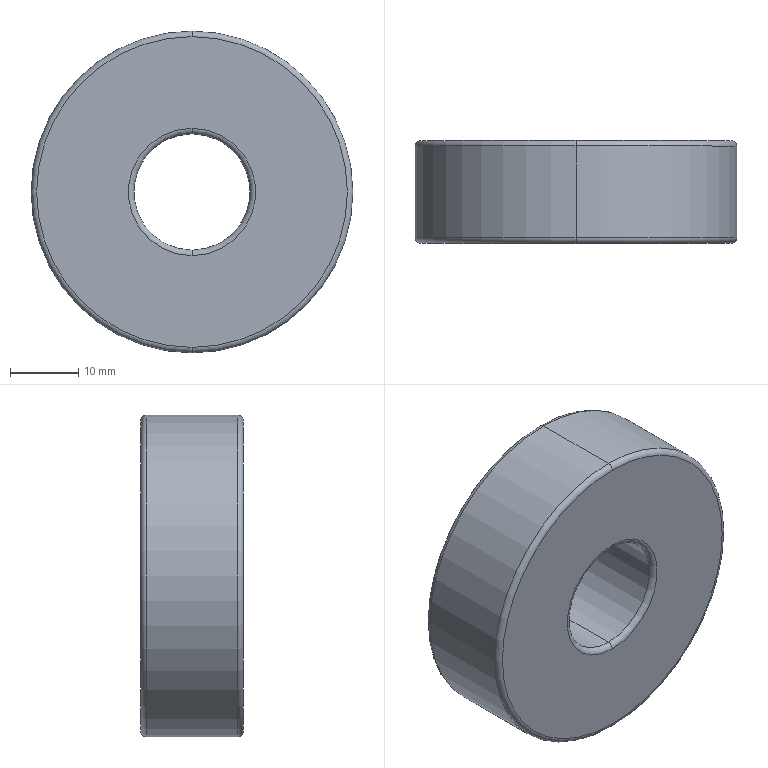Part | SolidWorks | features Extrusion 1, Fillet 1 | 1 solid | 14 faces | box 47 x 15 x 47 mm | volume 22564 mm3 | torus 8 | cylinder 4 | plane 2 | commonest cylinder face diameters 17 x2 47 x2
STEP:
#1=CARTESIAN_POINT('',(0.,14.2,-23.5));
#2=VERTEX_POINT('',#1);
#3=CARTESIAN_POINT('',(0.,14.2,23.5));
#4=VERTEX_POINT('',#3);
#5=CARTESIAN_POINT('',(0.,14.2,0.));
#6=DIRECTION('',(0.,-1.,0.));
#7=DIRECTION('',(0.,0.,1.));
#8=AXIS2_PLACEMENT_3D('',#5,#6,#7);
#9=CIRCLE('',#8,23.5);
#10=EDGE_CURVE('',#2,#4,#9,.T.);
#11=ORIENTED_EDGE('',*,*,#10,.F.);
#12=CARTESIAN_POINT('',(0.,15.,-22.7));
#13=VERTEX_POINT('',#12);
#14=CARTESIAN_POINT('',(0.,14.2,-22.7));
#15=DIRECTION('',(1.,0.,0.));
#16=DIRECTION('',(0.,0.,-1.));
#17=AXIS2_PLACEMENT_3D('',#14,#15,#16);
#18=CIRCLE('',#17,0.8);
#19=EDGE_CURVE('',#2,#13,#18,.T.);
#20=ORIENTED_EDGE('',*,*,#19,.T.);
#21=CARTESIAN_POINT('',(0.,15.,22.7));
#22=VERTEX_POINT('',#21);
#23=CARTESIAN_POINT('',(0.,15.,0.));
#24=DIRECTION('',(0.,1.,0.));
#25=DIRECTION('',(0.,0.,1.));
#26=AXIS2_PLACEMENT_3D('',#23,#24,#25);
#27=CIRCLE('',#26,22.7);
#28=EDGE_CURVE('',#22,#13,#27,.T.);
#29=ORIENTED_EDGE('',*,*,#28,.F.);
#30=CARTESIAN_POINT('',(0.,14.2,22.7));
#31=DIRECTION('',(-1.,0.,0.));
#32=DIRECTION('',(0.,0.,1.));
#33=AXIS2_PLACEMENT_3D('',#30,#31,#32);
#34=CIRCLE('',#33,0.8);
#35=EDGE_CURVE('',#4,#22,#34,.T.);
#36=ORIENTED_EDGE('',*,*,#35,.F.);
#37=EDGE_LOOP('',(#11,#20,#29,#36));
#38=FACE_OUTER_BOUND('',#37,.T.);
#39=CARTESIAN_POINT('',(0.,14.2,0.));
#40=DIRECTION('',(0.,1.,0.));
#41=DIRECTION('',(0.,0.,1.));
#42=AXIS2_PLACEMENT_3D('',#39,#40,#41);
#43=TOROIDAL_SURFACE('',#42,22.7,0.8);
#44=ADVANCED_FACE('',(#38),#43,.T.);
#45=CARTESIAN_POINT('',(0.,15.,-9.3));
#46=VERTEX_POINT('',#45);
#47=CARTESIAN_POINT('',(0.,15.,9.3));
#48=VERTEX_POINT('',#47);
#49=CARTESIAN_POINT('',(0.,15.,0.));
#50=DIRECTION('',(0.,-1.,0.));
#51=DIRECTION('',(0.,0.,1.));
#52=AXIS2_PLACEMENT_3D('',#49,#50,#51);
#53=CIRCLE('',#52,9.3);
#54=EDGE_CURVE('',#46,#48,#53,.T.);
#55=ORIENTED_EDGE('',*,*,#54,.F.);
#56=CARTESIAN_POINT('',(0.,14.2,-8.5));
#57=VERTEX_POINT('',#56);
#58=CARTESIAN_POINT('',(0.,14.2,-9.3));
#59=DIRECTION('',(1.,0.,0.));
#60=DIRECTION('',(0.,0.,-1.));
#61=AXIS2_PLACEMENT_3D('',#58,#59,#60);
#62=CIRCLE('',#61,0.8);
#63=EDGE_CURVE('',#46,#57,#62,.T.);
#64=ORIENTED_EDGE('',*,*,#63,.T.);
#65=CARTESIAN_POINT('',(0.,14.2,8.5));
#66=VERTEX_POINT('',#65);
#67=CARTESIAN_POINT('',(0.,14.2,0.));
#68=DIRECTION('',(0.,1.,0.));
#69=DIRECTION('',(0.,0.,1.));
#70=AXIS2_PLACEMENT_3D('',#67,#68,#69);
#71=CIRCLE('',#70,8.5);
#72=EDGE_CURVE('',#66,#57,#71,.T.);
#73=ORIENTED_EDGE('',*,*,#72,.F.);
#74=CARTESIAN_POINT('',(0.,14.2,9.3));
#75=DIRECTION('',(-1.,0.,0.));
#76=DIRECTION('',(0.,0.,1.));
#77=AXIS2_PLACEMENT_3D('',#74,#75,#76);
#78=CIRCLE('',#77,0.8);
#79=EDGE_CURVE('',#48,#66,#78,.T.);
#80=ORIENTED_EDGE('',*,*,#79,.F.);
#81=EDGE_LOOP('',(#55,#64,#73,#80));
#82=FACE_OUTER_BOUND('',#81,.T.);
#83=CARTESIAN_POINT('',(0.,14.2,0.));
#84=DIRECTION('',(0.,1.,0.));
#85=DIRECTION('',(0.,0.,1.));
#86=AXIS2_PLACEMENT_3D('',#83,#84,#85);
#87=TOROIDAL_SURFACE('',#86,9.3,0.8);
#88=ADVANCED_FACE('',(#82),#87,.T.);
#89=CARTESIAN_POINT('',(0.,0.,-22.7));
#90=VERTEX_POINT('',#89);
#91=CARTESIAN_POINT('',(0.,0.,22.7));
#92=VERTEX_POINT('',#91);
#93=CARTESIAN_POINT('',(0.,0.,0.));
#94=DIRECTION('',(0.,-1.,0.));
#95=DIRECTION('',(0.,0.,1.));
#96=AXIS2_PLACEMENT_3D('',#93,#94,#95);
#97=CIRCLE('',#96,22.7);
#98=EDGE_CURVE('',#90,#92,#97,.T.);
#99=ORIENTED_EDGE('',*,*,#98,.F.);
#100=CARTESIAN_POINT('',(0.,0.8,-23.5));
#101=VERTEX_POINT('',#100);
#102=CARTESIAN_POINT('',(0.,0.8,-22.7));
#103=DIRECTION('',(1.,0.,0.));
#104=DIRECTION('',(0.,0.,-1.));
#105=AXIS2_PLACEMENT_3D('',#102,#103,#104);
#106=CIRCLE('',#105,0.8);
#107=EDGE_CURVE('',#90,#101,#106,.T.);
#108=ORIENTED_EDGE('',*,*,#107,.T.);
#109=CARTESIAN_POINT('',(0.,0.8,23.5));
#110=VERTEX_POINT('',#109);
#111=CARTESIAN_POINT('',(0.,0.8,0.));
#112=DIRECTION('',(0.,1.,0.));
#113=DIRECTION('',(0.,0.,1.));
#114=AXIS2_PLACEMENT_3D('',#111,#112,#113);
#115=CIRCLE('',#114,23.5);
#116=EDGE_CURVE('',#110,#101,#115,.T.);
#117=ORIENTED_EDGE('',*,*,#116,.F.);
#118=CARTESIAN_POINT('',(0.,0.8,22.7));
#119=DIRECTION('',(-1.,0.,0.));
#120=DIRECTION('',(0.,0.,1.));
#121=AXIS2_PLACEMENT_3D('',#118,#119,#120);
#122=CIRCLE('',#121,0.8);
#123=EDGE_CURVE('',#92,#110,#122,.T.);
#124=ORIENTED_EDGE('',*,*,#123,.F.);
#125=EDGE_LOOP('',(#99,#108,#117,#124));
#126=FACE_OUTER_BOUND('',#125,.T.);
#127=CARTESIAN_POINT('',(0.,0.8,0.));
#128=DIRECTION('',(0.,1.,0.));
#129=DIRECTION('',(0.,0.,1.));
#130=AXIS2_PLACEMENT_3D('',#127,#128,#129);
#131=TOROIDAL_SURFACE('',#130,22.7,0.8);
#132=ADVANCED_FACE('',(#126),#131,.T.);
#133=CARTESIAN_POINT('',(0.,0.8,-8.5));
#134=VERTEX_POINT('',#133);
#135=CARTESIAN_POINT('',(0.,0.8,8.5));
#136=VERTEX_POINT('',#135);
#137=CARTESIAN_POINT('',(0.,0.8,0.));
#138=DIRECTION('',(0.,-1.,0.));
#139=DIRECTION('',(0.,0.,1.));
#140=AXIS2_PLACEMENT_3D('',#137,#138,#139);
#141=CIRCLE('',#140,8.5);
#142=EDGE_CURVE('',#134,#136,#141,.T.);
#143=ORIENTED_EDGE('',*,*,#142,.F.);
#144=CARTESIAN_POINT('',(0.,0.,-9.3));
#145=VERTEX_POINT('',#144);
#146=CARTESIAN_POINT('',(0.,0.8,-9.3));
#147=DIRECTION('',(1.,0.,0.));
#148=DIRECTION('',(0.,0.,-1.));
#149=AXIS2_PLACEMENT_3D('',#146,#147,#148);
#150=CIRCLE('',#149,0.8);
#151=EDGE_CURVE('',#134,#145,#150,.T.);
#152=ORIENTED_EDGE('',*,*,#151,.T.);
#153=CARTESIAN_POINT('',(0.,0.,9.3));
#154=VERTEX_POINT('',#153);
#155=CARTESIAN_POINT('',(0.,0.,0.));
#156=DIRECTION('',(0.,1.,0.));
#157=DIRECTION('',(0.,0.,1.));
#158=AXIS2_PLACEMENT_3D('',#155,#156,#157);
#159=CIRCLE('',#158,9.3);
#160=EDGE_CURVE('',#154,#145,#159,.T.);
#161=ORIENTED_EDGE('',*,*,#160,.F.);
#162=CARTESIAN_POINT('',(0.,0.8,9.3));
#163=DIRECTION('',(-1.,0.,0.));
#164=DIRECTION('',(0.,0.,1.));
#165=AXIS2_PLACEMENT_3D('',#162,#163,#164);
#166=CIRCLE('',#165,0.8);
#167=EDGE_CURVE('',#136,#154,#166,.T.);
#168=ORIENTED_EDGE('',*,*,#167,.F.);
#169=EDGE_LOOP('',(#143,#152,#161,#168));
#170=FACE_OUTER_BOUND('',#169,.T.);
#171=CARTESIAN_POINT('',(0.,0.8,0.));
#172=DIRECTION('',(0.,1.,0.));
#173=DIRECTION('',(0.,0.,1.));
#174=AXIS2_PLACEMENT_3D('',#171,#172,#173);
#175=TOROIDAL_SURFACE('',#174,9.3,0.8);
#176=ADVANCED_FACE('',(#170),#175,.T.);
#177=CARTESIAN_POINT('',(0.,14.2,0.));
#178=DIRECTION('',(0.,1.,0.));
#179=DIRECTION('',(0.,0.,1.));
#180=AXIS2_PLACEMENT_3D('',#177,#178,#179);
#181=CIRCLE('',#180,8.5);
#182=EDGE_CURVE('',#57,#66,#181,.T.);
#183=ORIENTED_EDGE('',*,*,#182,.T.);
#184=CARTESIAN_POINT('',(0.,15.,8.5));
#185=DIRECTION('',(0.,-1.,0.));
#186=VECTOR('',#185,1000.);
#187=LINE('',#184,#186);
#188=EDGE_CURVE('',#66,#136,#187,.T.);
#189=ORIENTED_EDGE('',*,*,#188,.T.);
#190=CARTESIAN_POINT('',(0.,0.8,0.));
#191=DIRECTION('',(0.,-1.,0.));
#192=DIRECTION('',(0.,0.,1.));
#193=AXIS2_PLACEMENT_3D('',#190,#191,#192);
#194=CIRCLE('',#193,8.5);
#195=EDGE_CURVE('',#136,#134,#194,.T.);
#196=ORIENTED_EDGE('',*,*,#195,.T.);
#197=CARTESIAN_POINT('',(0.,15.,-8.5));
#198=DIRECTION('',(0.,-1.,0.));
#199=VECTOR('',#198,1000.);
#200=LINE('',#197,#199);
#201=EDGE_CURVE('',#57,#134,#200,.T.);
#202=ORIENTED_EDGE('',*,*,#201,.F.);
#203=EDGE_LOOP('',(#183,#189,#196,#202));
#204=FACE_OUTER_BOUND('',#203,.T.);
#205=CARTESIAN_POINT('',(0.,15.,0.));
#206=DIRECTION('',(0.,-1.,0.));
#207=DIRECTION('',(0.,0.,-1.));
#208=AXIS2_PLACEMENT_3D('',#205,#206,#207);
#209=CYLINDRICAL_SURFACE('',#208,8.5);
#210=ADVANCED_FACE('',(#204),#209,.F.);
#211=ORIENTED_EDGE('',*,*,#10,.T.);
#212=CARTESIAN_POINT('',(0.,15.,23.5));
#213=DIRECTION('',(0.,-1.,0.));
#214=VECTOR('',#213,1000.);
#215=LINE('',#212,#214);
#216=EDGE_CURVE('',#4,#110,#215,.T.);
#217=ORIENTED_EDGE('',*,*,#216,.T.);
#218=ORIENTED_EDGE('',*,*,#116,.T.);
#219=CARTESIAN_POINT('',(0.,15.,-23.5));
#220=DIRECTION('',(0.,-1.,0.));
#221=VECTOR('',#220,1000.);
#222=LINE('',#219,#221);
#223=EDGE_CURVE('',#2,#101,#222,.T.);
#224=ORIENTED_EDGE('',*,*,#223,.F.);
#225=EDGE_LOOP('',(#211,#217,#218,#224));
#226=FACE_OUTER_BOUND('',#225,.T.);
#227=CARTESIAN_POINT('',(0.,15.,0.));
#228=DIRECTION('',(0.,-1.,0.));
#229=DIRECTION('',(0.,0.,-1.));
#230=AXIS2_PLACEMENT_3D('',#227,#228,#229);
#231=CYLINDRICAL_SURFACE('',#230,23.5);
#232=ADVANCED_FACE('',(#226),#231,.T.);
#233=CARTESIAN_POINT('',(0.,15.,0.));
#234=DIRECTION('',(0.,-1.,0.));
#235=DIRECTION('',(0.,0.,1.));
#236=AXIS2_PLACEMENT_3D('',#233,#234,#235);
#237=CIRCLE('',#236,9.3);
#238=EDGE_CURVE('',#48,#46,#237,.T.);
#239=ORIENTED_EDGE('',*,*,#238,.T.);
#240=ORIENTED_EDGE('',*,*,#54,.T.);
#241=EDGE_LOOP('',(#239,#240));
#242=FACE_BOUND('',#241,.T.);
#243=ORIENTED_EDGE('',*,*,#28,.T.);
#244=CARTESIAN_POINT('',(0.,15.,0.));
#245=DIRECTION('',(0.,1.,0.));
#246=DIRECTION('',(0.,0.,1.));
#247=AXIS2_PLACEMENT_3D('',#244,#245,#246);
#248=CIRCLE('',#247,22.7);
#249=EDGE_CURVE('',#13,#22,#248,.T.);
#250=ORIENTED_EDGE('',*,*,#249,.T.);
#251=EDGE_LOOP('',(#243,#250));
#252=FACE_OUTER_BOUND('',#251,.T.);
#253=CARTESIAN_POINT('',(0.,15.,0.));
#254=DIRECTION('',(0.,1.,0.));
#255=DIRECTION('',(0.,0.,1.));
#256=AXIS2_PLACEMENT_3D('',#253,#254,#255);
#257=PLANE('',#256);
#258=ADVANCED_FACE('',(#242,#252),#257,.T.);
#259=ORIENTED_EDGE('',*,*,#160,.T.);
#260=CARTESIAN_POINT('',(0.,0.,0.));
#261=DIRECTION('',(0.,1.,0.));
#262=DIRECTION('',(0.,0.,1.));
#263=AXIS2_PLACEMENT_3D('',#260,#261,#262);
#264=CIRCLE('',#263,9.3);
#265=EDGE_CURVE('',#145,#154,#264,.T.);
#266=ORIENTED_EDGE('',*,*,#265,.T.);
#267=EDGE_LOOP('',(#259,#266));
#268=FACE_BOUND('',#267,.T.);
#269=CARTESIAN_POINT('',(0.,0.,0.));
#270=DIRECTION('',(0.,-1.,0.));
#271=DIRECTION('',(0.,0.,1.));
#272=AXIS2_PLACEMENT_3D('',#269,#270,#271);
#273=CIRCLE('',#272,22.7);
#274=EDGE_CURVE('',#92,#90,#273,.T.);
#275=ORIENTED_EDGE('',*,*,#274,.T.);
#276=ORIENTED_EDGE('',*,*,#98,.T.);
#277=EDGE_LOOP('',(#275,#276));
#278=FACE_OUTER_BOUND('',#277,.T.);
#279=CARTESIAN_POINT('',(0.,0.,0.));
#280=DIRECTION('',(0.,1.,0.));
#281=DIRECTION('',(0.,0.,1.));
#282=AXIS2_PLACEMENT_3D('',#279,#280,#281);
#283=PLANE('',#282);
#284=ADVANCED_FACE('',(#268,#278),#283,.F.);
#285=ORIENTED_EDGE('',*,*,#216,.F.);
#286=CARTESIAN_POINT('',(0.,14.2,0.));
#287=DIRECTION('',(0.,-1.,0.));
#288=DIRECTION('',(0.,0.,1.));
#289=AXIS2_PLACEMENT_3D('',#286,#287,#288);
#290=CIRCLE('',#289,23.5);
#291=EDGE_CURVE('',#4,#2,#290,.T.);
#292=ORIENTED_EDGE('',*,*,#291,.T.);
#293=ORIENTED_EDGE('',*,*,#223,.T.);
#294=CARTESIAN_POINT('',(0.,0.8,0.));
#295=DIRECTION('',(0.,1.,0.));
#296=DIRECTION('',(0.,0.,1.));
#297=AXIS2_PLACEMENT_3D('',#294,#295,#296);
#298=CIRCLE('',#297,23.5);
#299=EDGE_CURVE('',#101,#110,#298,.T.);
#300=ORIENTED_EDGE('',*,*,#299,.T.);
#301=EDGE_LOOP('',(#285,#292,#293,#300));
#302=FACE_OUTER_BOUND('',#301,.T.);
#303=CARTESIAN_POINT('',(0.,15.,0.));
#304=DIRECTION('',(0.,-1.,0.));
#305=DIRECTION('',(0.,0.,-1.));
#306=AXIS2_PLACEMENT_3D('',#303,#304,#305);
#307=CYLINDRICAL_SURFACE('',#306,23.5);
#308=ADVANCED_FACE('',(#302),#307,.T.);
#309=ORIENTED_EDGE('',*,*,#188,.F.);
#310=ORIENTED_EDGE('',*,*,#72,.T.);
#311=ORIENTED_EDGE('',*,*,#201,.T.);
#312=ORIENTED_EDGE('',*,*,#142,.T.);
#313=EDGE_LOOP('',(#309,#310,#311,#312));
#314=FACE_OUTER_BOUND('',#313,.T.);
#315=CARTESIAN_POINT('',(0.,15.,0.));
#316=DIRECTION('',(0.,-1.,0.));
#317=DIRECTION('',(0.,0.,-1.));
#318=AXIS2_PLACEMENT_3D('',#315,#316,#317);
#319=CYLINDRICAL_SURFACE('',#318,8.5);
#320=ADVANCED_FACE('',(#314),#319,.F.);
#321=ORIENTED_EDGE('',*,*,#151,.F.);
#322=ORIENTED_EDGE('',*,*,#195,.F.);
#323=ORIENTED_EDGE('',*,*,#167,.T.);
#324=ORIENTED_EDGE('',*,*,#265,.F.);
#325=EDGE_LOOP('',(#321,#322,#323,#324));
#326=FACE_OUTER_BOUND('',#325,.T.);
#327=CARTESIAN_POINT('',(0.,0.8,0.));
#328=DIRECTION('',(0.,1.,0.));
#329=DIRECTION('',(0.,0.,1.));
#330=AXIS2_PLACEMENT_3D('',#327,#328,#329);
#331=TOROIDAL_SURFACE('',#330,9.3,0.8);
#332=ADVANCED_FACE('',(#326),#331,.T.);
#333=ORIENTED_EDGE('',*,*,#107,.F.);
#334=ORIENTED_EDGE('',*,*,#274,.F.);
#335=ORIENTED_EDGE('',*,*,#123,.T.);
#336=ORIENTED_EDGE('',*,*,#299,.F.);
#337=EDGE_LOOP('',(#333,#334,#335,#336));
#338=FACE_OUTER_BOUND('',#337,.T.);
#339=CARTESIAN_POINT('',(0.,0.8,0.));
#340=DIRECTION('',(0.,1.,0.));
#341=DIRECTION('',(0.,0.,1.));
#342=AXIS2_PLACEMENT_3D('',#339,#340,#341);
#343=TOROIDAL_SURFACE('',#342,22.7,0.8);
#344=ADVANCED_FACE('',(#338),#343,.T.);
#345=ORIENTED_EDGE('',*,*,#63,.F.);
#346=ORIENTED_EDGE('',*,*,#238,.F.);
#347=ORIENTED_EDGE('',*,*,#79,.T.);
#348=ORIENTED_EDGE('',*,*,#182,.F.);
#349=EDGE_LOOP('',(#345,#346,#347,#348));
#350=FACE_OUTER_BOUND('',#349,.T.);
#351=CARTESIAN_POINT('',(0.,14.2,0.));
#352=DIRECTION('',(0.,1.,0.));
#353=DIRECTION('',(0.,0.,1.));
#354=AXIS2_PLACEMENT_3D('',#351,#352,#353);
#355=TOROIDAL_SURFACE('',#354,9.3,0.8);
#356=ADVANCED_FACE('',(#350),#355,.T.);
#357=ORIENTED_EDGE('',*,*,#19,.F.);
#358=ORIENTED_EDGE('',*,*,#291,.F.);
#359=ORIENTED_EDGE('',*,*,#35,.T.);
#360=ORIENTED_EDGE('',*,*,#249,.F.);
#361=EDGE_LOOP('',(#357,#358,#359,#360));
#362=FACE_OUTER_BOUND('',#361,.T.);
#363=CARTESIAN_POINT('',(0.,14.2,0.));
#364=DIRECTION('',(0.,1.,0.));
#365=DIRECTION('',(0.,0.,1.));
#366=AXIS2_PLACEMENT_3D('',#363,#364,#365);
#367=TOROIDAL_SURFACE('',#366,22.7,0.8);
#368=ADVANCED_FACE('',(#362),#367,.T.);
#369=CLOSED_SHELL('',(#44,#88,#132,#176,#210,#232,#258,#284,#308,#320,#332,#344,#356,#368));
#370=MANIFOLD_SOLID_BREP('',#369);
#371=CARTESIAN_POINT('',(0.,0.,0.));
#372=DIRECTION('',(0.,0.,1.));
#373=DIRECTION('',(1.,0.,0.));
#374=AXIS2_PLACEMENT_3D('',#371,#372,#373);
#375=(LENGTH_UNIT()NAMED_UNIT(*)SI_UNIT(.MILLI.,.METRE.));
#376=UNCERTAINTY_MEASURE_WITH_UNIT(LENGTH_MEASURE(0.00001),#375,'','');
#377=(NAMED_UNIT(*)PLANE_ANGLE_UNIT()SI_UNIT($,.RADIAN.));
#378=(NAMED_UNIT(*)SI_UNIT($,.STERADIAN.)SOLID_ANGLE_UNIT());
#379=(GEOMETRIC_REPRESENTATION_CONTEXT(3)GLOBAL_UNCERTAINTY_ASSIGNED_CONTEXT((#376))GLOBAL_UNIT_ASSIGNED_CONTEXT((#375,#377,#378))REPRESENTATION_CONTEXT('',''));
#380=ADVANCED_BREP_SHAPE_REPRESENTATION('',(#370,#374),#379);